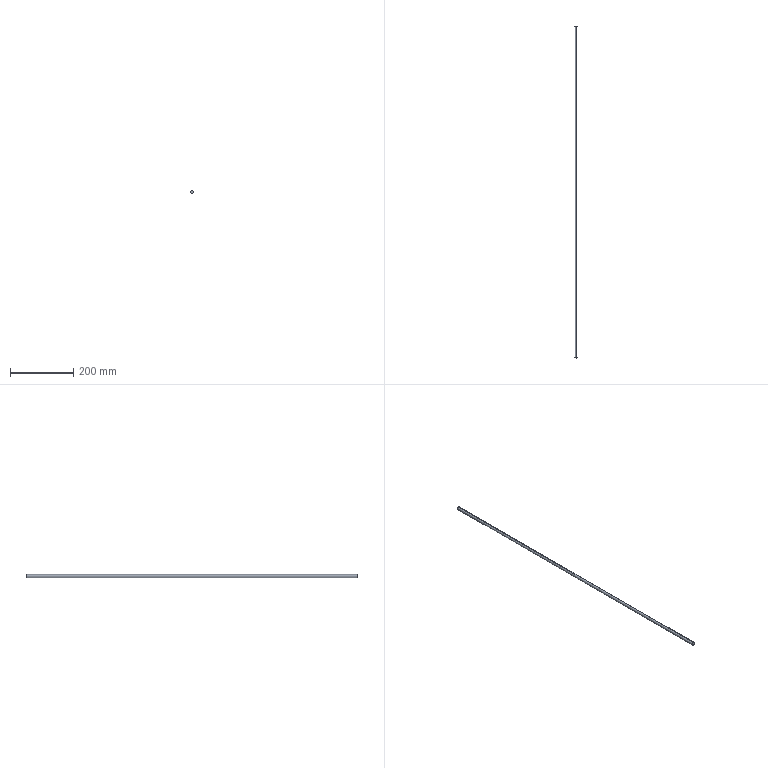Part | STEP file | 4-20.sldasm-Part-138 | 1 solid | 4 faces | box 9.525 x 1050 x 9.525 mm | volume 74819 mm3 | cylinder 2 | plane 2 | commonest cylinder face diameters 9.525 x2
STEP:
#1=CARTESIAN_POINT('',(143.125,525.,48.762));
#2=VERTEX_POINT('',#1);
#3=CARTESIAN_POINT('',(143.125,525.,39.237));
#4=VERTEX_POINT('',#3);
#5=CARTESIAN_POINT('',(143.125,525.,44.));
#6=DIRECTION('',(0.,1.,0.));
#7=DIRECTION('',(0.,0.,1.));
#8=AXIS2_PLACEMENT_3D('',#5,#6,#7);
#9=CIRCLE('',#8,4.763);
#10=EDGE_CURVE('',#2,#4,#9,.T.);
#11=ORIENTED_EDGE('',*,*,#10,.F.);
#12=CARTESIAN_POINT('',(143.125,-525.,48.762));
#13=VERTEX_POINT('',#12);
#14=CARTESIAN_POINT('',(143.125,431.8,48.762));
#15=DIRECTION('',(0.,-1.,0.));
#16=VECTOR('',#15,1000.);
#17=LINE('',#14,#16);
#18=EDGE_CURVE('',#2,#13,#17,.T.);
#19=ORIENTED_EDGE('',*,*,#18,.T.);
#20=CARTESIAN_POINT('',(143.125,-525.,39.237));
#21=VERTEX_POINT('',#20);
#22=CARTESIAN_POINT('',(143.125,-525.,44.));
#23=DIRECTION('',(0.,1.,0.));
#24=DIRECTION('',(0.,0.,-1.));
#25=AXIS2_PLACEMENT_3D('',#22,#23,#24);
#26=CIRCLE('',#25,4.763);
#27=EDGE_CURVE('',#13,#21,#26,.T.);
#28=ORIENTED_EDGE('',*,*,#27,.T.);
#29=CARTESIAN_POINT('',(143.125,431.8,39.237));
#30=DIRECTION('',(0.,-1.,0.));
#31=VECTOR('',#30,1000.);
#32=LINE('',#29,#31);
#33=EDGE_CURVE('',#4,#21,#32,.T.);
#34=ORIENTED_EDGE('',*,*,#33,.F.);
#35=EDGE_LOOP('',(#11,#19,#28,#34));
#36=FACE_OUTER_BOUND('',#35,.T.);
#37=CARTESIAN_POINT('',(143.125,431.8,44.));
#38=DIRECTION('',(0.,-1.,0.));
#39=DIRECTION('',(0.,0.,-1.));
#40=AXIS2_PLACEMENT_3D('',#37,#38,#39);
#41=CYLINDRICAL_SURFACE('',#40,4.763);
#42=ADVANCED_FACE('',(#36),#41,.T.);
#43=ORIENTED_EDGE('',*,*,#18,.F.);
#44=CARTESIAN_POINT('',(143.125,525.,44.));
#45=DIRECTION('',(0.,1.,0.));
#46=DIRECTION('',(0.,0.,1.));
#47=AXIS2_PLACEMENT_3D('',#44,#45,#46);
#48=CIRCLE('',#47,4.763);
#49=EDGE_CURVE('',#4,#2,#48,.T.);
#50=ORIENTED_EDGE('',*,*,#49,.F.);
#51=ORIENTED_EDGE('',*,*,#33,.T.);
#52=CARTESIAN_POINT('',(143.125,-525.,44.));
#53=DIRECTION('',(0.,1.,0.));
#54=DIRECTION('',(0.,0.,-1.));
#55=AXIS2_PLACEMENT_3D('',#52,#53,#54);
#56=CIRCLE('',#55,4.763);
#57=EDGE_CURVE('',#21,#13,#56,.T.);
#58=ORIENTED_EDGE('',*,*,#57,.T.);
#59=EDGE_LOOP('',(#43,#50,#51,#58));
#60=FACE_OUTER_BOUND('',#59,.T.);
#61=CARTESIAN_POINT('',(143.125,431.8,44.));
#62=DIRECTION('',(0.,-1.,0.));
#63=DIRECTION('',(0.,0.,-1.));
#64=AXIS2_PLACEMENT_3D('',#61,#62,#63);
#65=CYLINDRICAL_SURFACE('',#64,4.763);
#66=ADVANCED_FACE('',(#60),#65,.T.);
#67=ORIENTED_EDGE('',*,*,#49,.T.);
#68=ORIENTED_EDGE('',*,*,#10,.T.);
#69=EDGE_LOOP('',(#67,#68));
#70=FACE_OUTER_BOUND('',#69,.T.);
#71=CARTESIAN_POINT('',(-212.5,525.,689.));
#72=DIRECTION('',(0.,1.,0.));
#73=DIRECTION('',(0.,0.,1.));
#74=AXIS2_PLACEMENT_3D('',#71,#72,#73);
#75=PLANE('',#74);
#76=ADVANCED_FACE('',(#70),#75,.T.);
#77=ORIENTED_EDGE('',*,*,#57,.F.);
#78=ORIENTED_EDGE('',*,*,#27,.F.);
#79=EDGE_LOOP('',(#77,#78));
#80=FACE_OUTER_BOUND('',#79,.T.);
#81=CARTESIAN_POINT('',(182.5,-525.,689.));
#82=DIRECTION('',(0.,-1.,0.));
#83=DIRECTION('',(0.,0.,-1.));
#84=AXIS2_PLACEMENT_3D('',#81,#82,#83);
#85=PLANE('',#84);
#86=ADVANCED_FACE('',(#80),#85,.T.);
#87=CLOSED_SHELL('',(#42,#66,#76,#86));
#88=MANIFOLD_SOLID_BREP('',#87);
#89=CARTESIAN_POINT('',(0.,0.,0.));
#90=DIRECTION('',(0.,0.,1.));
#91=DIRECTION('',(1.,0.,0.));
#92=AXIS2_PLACEMENT_3D('',#89,#90,#91);
#93=(LENGTH_UNIT()NAMED_UNIT(*)SI_UNIT(.MILLI.,.METRE.));
#94=UNCERTAINTY_MEASURE_WITH_UNIT(LENGTH_MEASURE(0.00001),#93,'','');
#95=(NAMED_UNIT(*)PLANE_ANGLE_UNIT()SI_UNIT($,.RADIAN.));
#96=(NAMED_UNIT(*)SI_UNIT($,.STERADIAN.)SOLID_ANGLE_UNIT());
#97=(GEOMETRIC_REPRESENTATION_CONTEXT(3)GLOBAL_UNCERTAINTY_ASSIGNED_CONTEXT((#94))GLOBAL_UNIT_ASSIGNED_CONTEXT((#93,#95,#96))REPRESENTATION_CONTEXT('',''));
#98=ADVANCED_BREP_SHAPE_REPRESENTATION('',(#88,#92),#97);